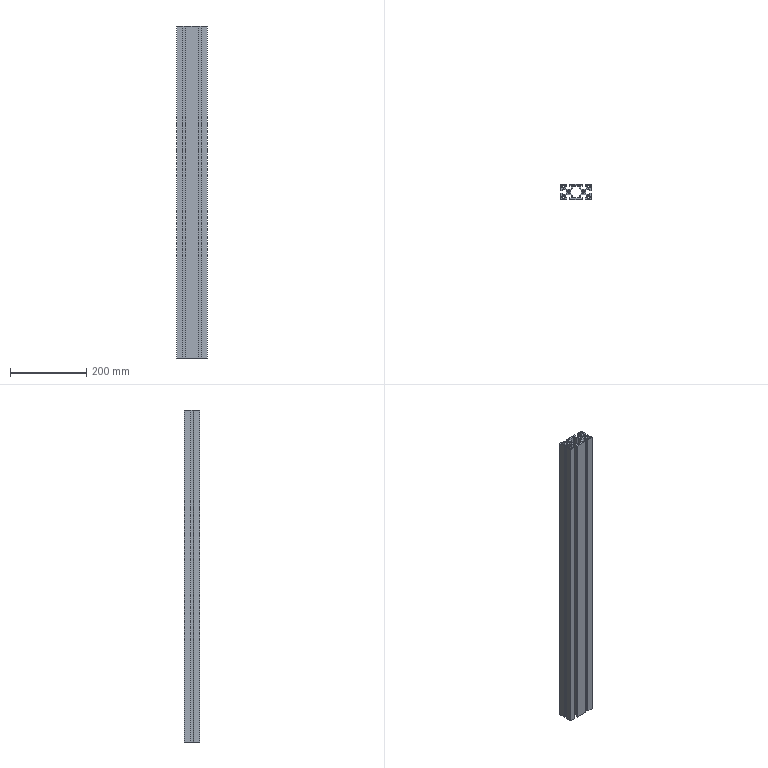Part | NX | 1 solid | 88 faces | box 80 x 40 x 871 mm | volume 1055196 mm3 | plane 78 | cylinder 10 | commonest cylinder face diameters 6 x4 8 x4 6.75 x2